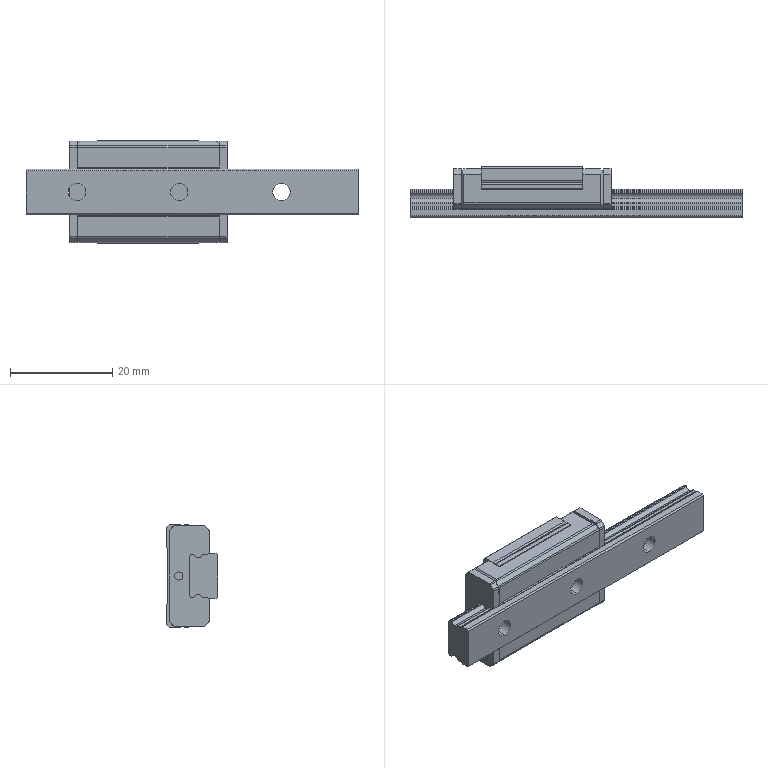Part | SolidWorks | 2 solids | 190 faces | box 65 x 10 x 20 mm | volume 6401 mm3 | plane 107 | cylinder 67 | cone 16 | commonest cylinder face diameters 1 x17 0.6 x12 0.3 x8 2.459 x8 2 x6 3.4 x6